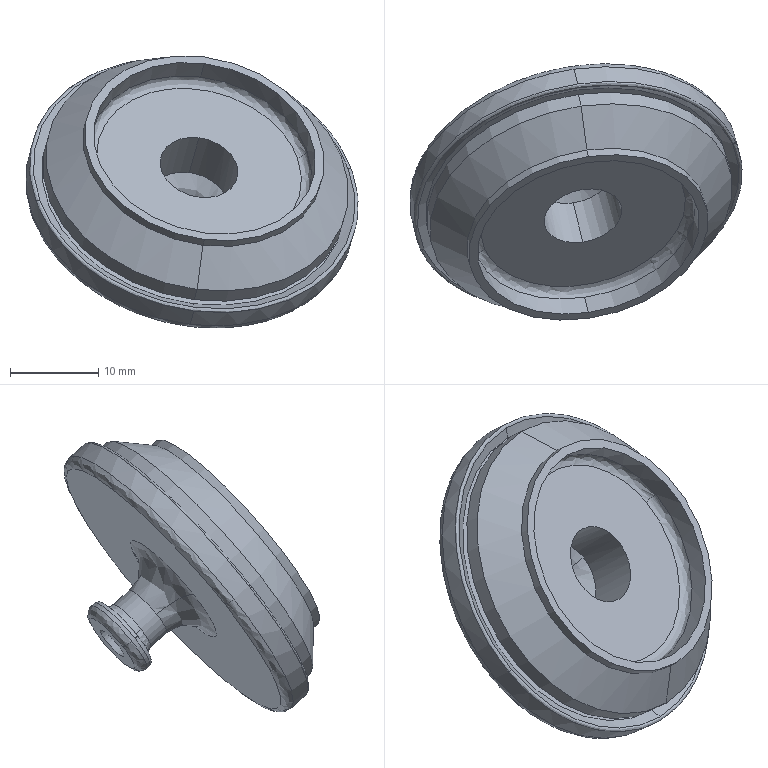Part | STEP file | PN_0005 | 1 solid | 45 faces | box 37.79 x 29.078 x 30.931 mm | volume 7006 mm3 | cylinder 18 | spline 16 | plane 7 | cone 4 | commonest cylinder face diameters 4 x2 6.4 x2 9 x2 9.5 x2 25.7 x2 27.7 x2